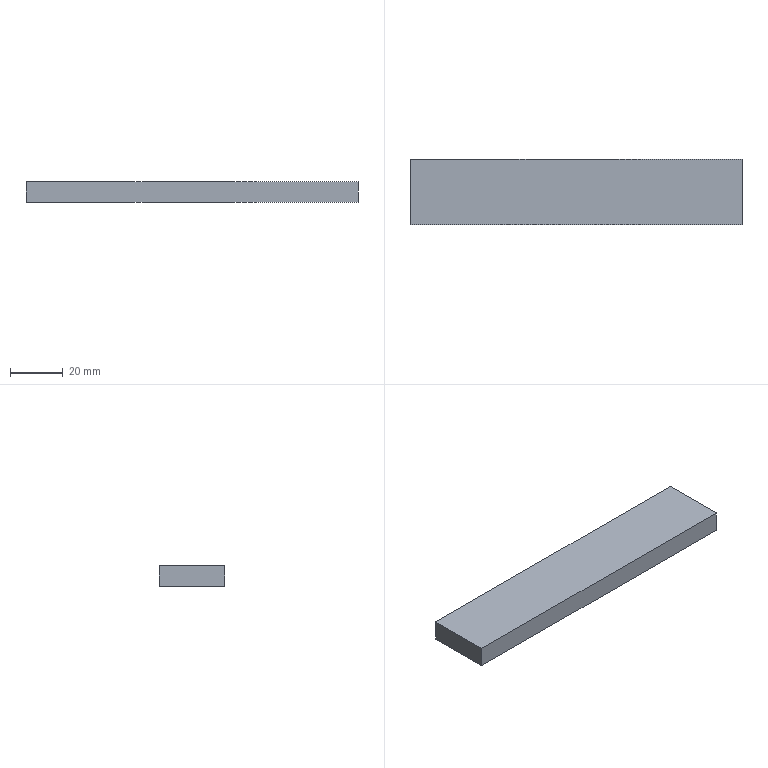Part | STEP file | Spacer block | 1 solid | 6 faces | box 126 x 24.75 x 7.95 mm | volume 24792 mm3 | plane 6
STEP:
#1=CARTESIAN_POINT('',(126.,195.742,7.95));
#2=VERTEX_POINT('',#1);
#3=CARTESIAN_POINT('',(126.,220.492,7.95));
#4=VERTEX_POINT('',#3);
#5=CARTESIAN_POINT('',(126.,195.742,7.95));
#6=DIRECTION('',(0.,1.,0.));
#7=VECTOR('',#6,1000.);
#8=LINE('',#5,#7);
#9=EDGE_CURVE('',#2,#4,#8,.T.);
#10=ORIENTED_EDGE('',*,*,#9,.F.);
#11=CARTESIAN_POINT('',(126.,195.742,0.));
#12=VERTEX_POINT('',#11);
#13=CARTESIAN_POINT('',(126.,195.742,136.358));
#14=DIRECTION('',(0.,0.,-1.));
#15=VECTOR('',#14,1000.);
#16=LINE('',#13,#15);
#17=EDGE_CURVE('',#2,#12,#16,.T.);
#18=ORIENTED_EDGE('',*,*,#17,.T.);
#19=CARTESIAN_POINT('',(126.,220.492,0.));
#20=VERTEX_POINT('',#19);
#21=CARTESIAN_POINT('',(126.,195.742,0.));
#22=DIRECTION('',(0.,1.,0.));
#23=VECTOR('',#22,1000.);
#24=LINE('',#21,#23);
#25=EDGE_CURVE('',#12,#20,#24,.T.);
#26=ORIENTED_EDGE('',*,*,#25,.T.);
#27=CARTESIAN_POINT('',(126.,220.492,136.358));
#28=DIRECTION('',(0.,0.,-1.));
#29=VECTOR('',#28,1000.);
#30=LINE('',#27,#29);
#31=EDGE_CURVE('',#4,#20,#30,.T.);
#32=ORIENTED_EDGE('',*,*,#31,.F.);
#33=EDGE_LOOP('',(#10,#18,#26,#32));
#34=FACE_OUTER_BOUND('',#33,.T.);
#35=CARTESIAN_POINT('',(126.,195.742,136.358));
#36=DIRECTION('',(-1.,0.,0.));
#37=DIRECTION('',(0.,0.,1.));
#38=AXIS2_PLACEMENT_3D('',#35,#36,#37);
#39=PLANE('',#38);
#40=ADVANCED_FACE('',(#34),#39,.F.);
#41=CARTESIAN_POINT('',(0.,220.492,7.95));
#42=VERTEX_POINT('',#41);
#43=CARTESIAN_POINT('',(126.,220.492,7.95));
#44=DIRECTION('',(-1.,0.,0.));
#45=VECTOR('',#44,1000.);
#46=LINE('',#43,#45);
#47=EDGE_CURVE('',#4,#42,#46,.T.);
#48=ORIENTED_EDGE('',*,*,#47,.F.);
#49=ORIENTED_EDGE('',*,*,#31,.T.);
#50=CARTESIAN_POINT('',(0.,220.492,0.));
#51=VERTEX_POINT('',#50);
#52=CARTESIAN_POINT('',(126.,220.492,0.));
#53=DIRECTION('',(-1.,0.,0.));
#54=VECTOR('',#53,1000.);
#55=LINE('',#52,#54);
#56=EDGE_CURVE('',#20,#51,#55,.T.);
#57=ORIENTED_EDGE('',*,*,#56,.T.);
#58=CARTESIAN_POINT('',(0.,220.492,136.358));
#59=DIRECTION('',(0.,0.,-1.));
#60=VECTOR('',#59,1000.);
#61=LINE('',#58,#60);
#62=EDGE_CURVE('',#42,#51,#61,.T.);
#63=ORIENTED_EDGE('',*,*,#62,.F.);
#64=EDGE_LOOP('',(#48,#49,#57,#63));
#65=FACE_OUTER_BOUND('',#64,.T.);
#66=CARTESIAN_POINT('',(126.,220.492,136.358));
#67=DIRECTION('',(0.,-1.,0.));
#68=DIRECTION('',(1.,0.,0.));
#69=AXIS2_PLACEMENT_3D('',#66,#67,#68);
#70=PLANE('',#69);
#71=ADVANCED_FACE('',(#65),#70,.F.);
#72=CARTESIAN_POINT('',(0.,195.742,7.95));
#73=VERTEX_POINT('',#72);
#74=CARTESIAN_POINT('',(0.,195.742,7.95));
#75=DIRECTION('',(0.,-1.,0.));
#76=VECTOR('',#75,1000.);
#77=LINE('',#74,#76);
#78=EDGE_CURVE('',#42,#73,#77,.T.);
#79=ORIENTED_EDGE('',*,*,#78,.F.);
#80=ORIENTED_EDGE('',*,*,#62,.T.);
#81=CARTESIAN_POINT('',(0.,195.742,0.));
#82=VERTEX_POINT('',#81);
#83=CARTESIAN_POINT('',(0.,195.742,0.));
#84=DIRECTION('',(0.,-1.,0.));
#85=VECTOR('',#84,1000.);
#86=LINE('',#83,#85);
#87=EDGE_CURVE('',#51,#82,#86,.T.);
#88=ORIENTED_EDGE('',*,*,#87,.T.);
#89=CARTESIAN_POINT('',(0.,195.742,136.358));
#90=DIRECTION('',(0.,0.,-1.));
#91=VECTOR('',#90,1000.);
#92=LINE('',#89,#91);
#93=EDGE_CURVE('',#73,#82,#92,.T.);
#94=ORIENTED_EDGE('',*,*,#93,.F.);
#95=EDGE_LOOP('',(#79,#80,#88,#94));
#96=FACE_OUTER_BOUND('',#95,.T.);
#97=CARTESIAN_POINT('',(0.,195.742,136.358));
#98=DIRECTION('',(1.,0.,0.));
#99=DIRECTION('',(0.,1.,0.));
#100=AXIS2_PLACEMENT_3D('',#97,#98,#99);
#101=PLANE('',#100);
#102=ADVANCED_FACE('',(#96),#101,.F.);
#103=CARTESIAN_POINT('',(126.,195.742,7.95));
#104=DIRECTION('',(1.,0.,0.));
#105=VECTOR('',#104,1000.);
#106=LINE('',#103,#105);
#107=EDGE_CURVE('',#73,#2,#106,.T.);
#108=ORIENTED_EDGE('',*,*,#107,.F.);
#109=ORIENTED_EDGE('',*,*,#93,.T.);
#110=CARTESIAN_POINT('',(126.,195.742,0.));
#111=DIRECTION('',(1.,0.,0.));
#112=VECTOR('',#111,1000.);
#113=LINE('',#110,#112);
#114=EDGE_CURVE('',#82,#12,#113,.T.);
#115=ORIENTED_EDGE('',*,*,#114,.T.);
#116=ORIENTED_EDGE('',*,*,#17,.F.);
#117=EDGE_LOOP('',(#108,#109,#115,#116));
#118=FACE_OUTER_BOUND('',#117,.T.);
#119=CARTESIAN_POINT('',(126.,195.742,136.358));
#120=DIRECTION('',(0.,1.,0.));
#121=DIRECTION('',(-1.,0.,0.));
#122=AXIS2_PLACEMENT_3D('',#119,#120,#121);
#123=PLANE('',#122);
#124=ADVANCED_FACE('',(#118),#123,.F.);
#125=ORIENTED_EDGE('',*,*,#25,.F.);
#126=ORIENTED_EDGE('',*,*,#114,.F.);
#127=ORIENTED_EDGE('',*,*,#87,.F.);
#128=ORIENTED_EDGE('',*,*,#56,.F.);
#129=EDGE_LOOP('',(#125,#126,#127,#128));
#130=FACE_OUTER_BOUND('',#129,.T.);
#131=CARTESIAN_POINT('',(0.,0.,0.));
#132=DIRECTION('',(0.,0.,1.));
#133=DIRECTION('',(1.,0.,0.));
#134=AXIS2_PLACEMENT_3D('',#131,#132,#133);
#135=PLANE('',#134);
#136=ADVANCED_FACE('',(#130),#135,.F.);
#137=ORIENTED_EDGE('',*,*,#107,.T.);
#138=ORIENTED_EDGE('',*,*,#9,.T.);
#139=ORIENTED_EDGE('',*,*,#47,.T.);
#140=ORIENTED_EDGE('',*,*,#78,.T.);
#141=EDGE_LOOP('',(#137,#138,#139,#140));
#142=FACE_OUTER_BOUND('',#141,.T.);
#143=CARTESIAN_POINT('',(0.,220.492,7.95));
#144=DIRECTION('',(0.,0.,1.));
#145=DIRECTION('',(1.,0.,0.));
#146=AXIS2_PLACEMENT_3D('',#143,#144,#145);
#147=PLANE('',#146);
#148=ADVANCED_FACE('',(#142),#147,.T.);
#149=CLOSED_SHELL('',(#40,#71,#102,#124,#136,#148));
#150=MANIFOLD_SOLID_BREP('',#149);
#151=CARTESIAN_POINT('',(0.,0.,0.));
#152=DIRECTION('',(0.,0.,1.));
#153=DIRECTION('',(1.,0.,0.));
#154=AXIS2_PLACEMENT_3D('',#151,#152,#153);
#155=(LENGTH_UNIT()NAMED_UNIT(*)SI_UNIT(.MILLI.,.METRE.));
#156=UNCERTAINTY_MEASURE_WITH_UNIT(LENGTH_MEASURE(0.00001),#155,'','');
#157=(NAMED_UNIT(*)PLANE_ANGLE_UNIT()SI_UNIT($,.RADIAN.));
#158=(NAMED_UNIT(*)SI_UNIT($,.STERADIAN.)SOLID_ANGLE_UNIT());
#159=(GEOMETRIC_REPRESENTATION_CONTEXT(3)GLOBAL_UNCERTAINTY_ASSIGNED_CONTEXT((#156))GLOBAL_UNIT_ASSIGNED_CONTEXT((#155,#157,#158))REPRESENTATION_CONTEXT('',''));
#160=ADVANCED_BREP_SHAPE_REPRESENTATION('',(#150,#154),#159);